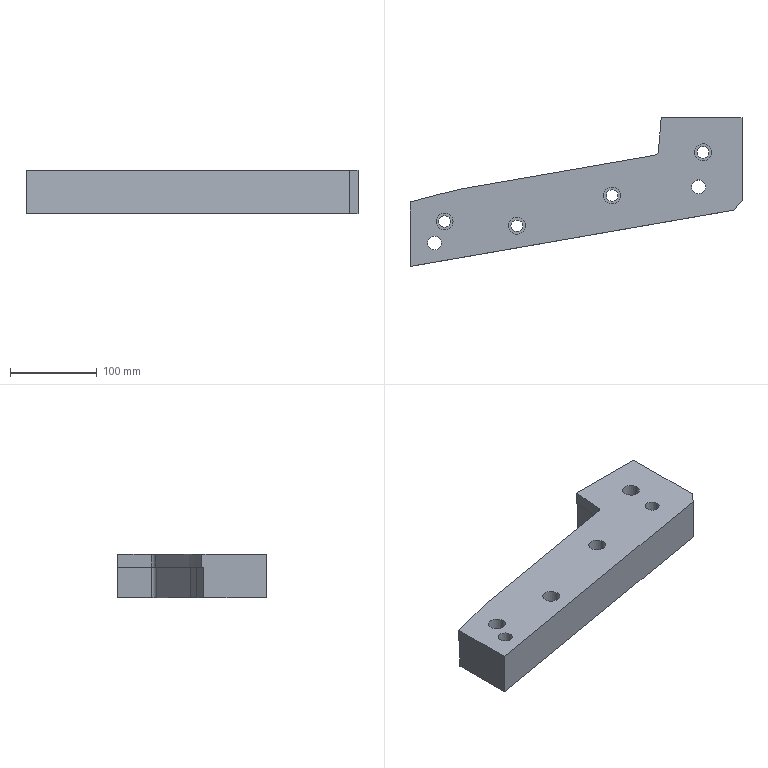Part | NX | features solid 2 | 1 solid | 31 faces | box 383.358 x 171.888 x 50 mm | volume 1583824 mm3 | plane 14 | cylinder 12 | spline 5 | commonest cylinder face diameters 13.5 x4 19.5 x4 16 x2 10 x1 14 x1
STEP:
#1=CARTESIAN_POINT('',(-1203.358,330.489,-15.));
#2=VERTEX_POINT('',#1);
#3=CARTESIAN_POINT('',(-1203.358,330.489,-50.));
#4=VERTEX_POINT('',#3);
#5=CARTESIAN_POINT('',(-1203.358,330.489,-32.5));
#6=DIRECTION('',(0.,0.,-1.));
#7=VECTOR('',#6,1000.);
#8=LINE('',#5,#7);
#9=EDGE_CURVE('',#2,#4,#8,.T.);
#10=ORIENTED_EDGE('',*,*,#9,.T.);
#11=CARTESIAN_POINT('',(-1203.358,258.112,-50.));
#12=VERTEX_POINT('',#11);
#13=CARTESIAN_POINT('',(-1203.358,307.899,-50.));
#14=DIRECTION('',(0.,-1.,0.));
#15=VECTOR('',#14,1000.);
#16=LINE('',#13,#15);
#17=EDGE_CURVE('',#4,#12,#16,.T.);
#18=ORIENTED_EDGE('',*,*,#17,.T.);
#19=CARTESIAN_POINT('',(-1203.358,258.112,0.));
#20=VERTEX_POINT('',#19);
#21=CARTESIAN_POINT('',(-1203.358,258.112,-50.));
#22=DIRECTION('',(0.,0.,1.));
#23=VECTOR('',#22,1000.);
#24=LINE('',#21,#23);
#25=EDGE_CURVE('',#12,#20,#24,.T.);
#26=ORIENTED_EDGE('',*,*,#25,.T.);
#27=CARTESIAN_POINT('',(-1203.358,332.538,0.));
#28=VERTEX_POINT('',#27);
#29=CARTESIAN_POINT('',(-1203.358,307.899,0.));
#30=DIRECTION('',(0.,-1.,0.));
#31=VECTOR('',#30,1000.);
#32=LINE('',#29,#31);
#33=EDGE_CURVE('',#28,#20,#32,.T.);
#34=ORIENTED_EDGE('',*,*,#33,.F.);
#35=CARTESIAN_POINT('',(-1203.358,332.538,-15.));
#36=VERTEX_POINT('',#35);
#37=CARTESIAN_POINT('',(-1203.358,332.538,0.));
#38=DIRECTION('',(0.,0.,1.));
#39=VECTOR('',#38,1000.);
#40=LINE('',#37,#39);
#41=EDGE_CURVE('',#28,#36,#40,.F.);
#42=ORIENTED_EDGE('',*,*,#41,.T.);
#43=CARTESIAN_POINT('',(-1203.358,390.837,-15.));
#44=DIRECTION('',(0.,-1.,0.));
#45=VECTOR('',#44,1000.);
#46=LINE('',#43,#45);
#47=EDGE_CURVE('',#2,#36,#46,.F.);
#48=ORIENTED_EDGE('',*,*,#47,.F.);
#49=EDGE_LOOP('',(#10,#18,#26,#34,#42,#48));
#50=FACE_BOUND('',#49,.T.);
#51=CARTESIAN_POINT('',(-1203.358,250.,0.));
#52=DIRECTION('',(1.,0.,0.));
#53=DIRECTION('',(0.,0.,-1.));
#54=AXIS2_PLACEMENT_3D('',#51,#52,#53);
#55=PLANE('',#54);
#56=ADVANCED_FACE('',(#50),#55,.F.);
#57=CARTESIAN_POINT('',(-1144.675,345.418,-15.));
#58=VERTEX_POINT('',#57);
#59=CARTESIAN_POINT('',(-1144.675,345.418,-50.));
#60=VERTEX_POINT('',#59);
#61=CARTESIAN_POINT('',(-1144.675,345.418,-65.));
#62=DIRECTION('',(0.,0.,-1.));
#63=VECTOR('',#62,1000.);
#64=LINE('',#61,#63);
#65=EDGE_CURVE('',#58,#60,#64,.T.);
#66=ORIENTED_EDGE('',*,*,#65,.F.);
#67=CARTESIAN_POINT('',(-920.081,384.447,-15.));
#68=VERTEX_POINT('',#67);
#69=CARTESIAN_POINT('',(-1144.675,345.418,-15.));
#70=CARTESIAN_POINT('',(-1107.244,351.927,-15.));
#71=CARTESIAN_POINT('',(-1051.098,361.701,-15.));
#72=CARTESIAN_POINT('',(-976.23,374.696,-15.));
#73=CARTESIAN_POINT('',(-938.808,381.26,-15.));
#74=CARTESIAN_POINT('',(-920.081,384.447,-15.));
#75=B_SPLINE_CURVE_WITH_KNOTS('',3,(#69,#70,#71,#72,#73,#74),.UNSPECIFIED.,.F.,.F.,(4,1,1,4),(0.07597,0.19,0.2469,0.3039),.UNSPECIFIED.);
#76=EDGE_CURVE('',#58,#68,#75,.T.);
#77=ORIENTED_EDGE('',*,*,#76,.T.);
#78=CARTESIAN_POINT('',(-920.081,384.446,-50.));
#79=VERTEX_POINT('',#78);
#80=CARTESIAN_POINT('',(-920.081,384.447,-32.5));
#81=DIRECTION('',(0.,0.,1.));
#82=VECTOR('',#81,1000.);
#83=LINE('',#80,#82);
#84=EDGE_CURVE('',#79,#68,#83,.T.);
#85=ORIENTED_EDGE('',*,*,#84,.F.);
#86=CARTESIAN_POINT('',(-920.081,384.447,-50.));
#87=CARTESIAN_POINT('',(-938.808,381.26,-50.));
#88=CARTESIAN_POINT('',(-976.23,374.696,-50.));
#89=CARTESIAN_POINT('',(-1051.098,361.701,-50.));
#90=CARTESIAN_POINT('',(-1107.244,351.927,-50.));
#91=CARTESIAN_POINT('',(-1144.675,345.418,-50.));
#92=B_SPLINE_CURVE_WITH_KNOTS('',3,(#86,#87,#88,#89,#90,#91),.UNSPECIFIED.,.F.,.F.,(4,1,1,4),(0.008531,0.06552,0.1225,0.2365),.UNSPECIFIED.);
#93=EDGE_CURVE('',#79,#60,#92,.T.);
#94=ORIENTED_EDGE('',*,*,#93,.T.);
#95=EDGE_LOOP('',(#66,#77,#85,#94));
#96=FACE_BOUND('',#95,.T.);
#97=CARTESIAN_POINT('',(-1144.675,345.418,-50.));
#98=CARTESIAN_POINT('',(-1144.675,345.418,-15.));
#99=CARTESIAN_POINT('',(-1107.243,351.928,-50.));
#100=CARTESIAN_POINT('',(-1107.243,351.928,-15.));
#101=CARTESIAN_POINT('',(-1051.094,361.702,-50.));
#102=CARTESIAN_POINT('',(-1051.094,361.702,-15.));
#103=CARTESIAN_POINT('',(-976.227,374.697,-50.));
#104=CARTESIAN_POINT('',(-976.227,374.697,-15.));
#105=CARTESIAN_POINT('',(-938.797,381.262,-50.));
#106=CARTESIAN_POINT('',(-938.797,381.262,-15.));
#107=CARTESIAN_POINT('',(-920.081,384.447,-50.));
#108=CARTESIAN_POINT('',(-920.081,384.447,-15.));
#109=B_SPLINE_SURFACE_WITH_KNOTS('',3,1,((#97,#98),(#99,#100),(#101,#102),(#103,#104),(#105,#106),(#107,#108)),.SURF_OF_LINEAR_EXTRUSION.,.F.,.F.,.F.,(4,1,1,4),(2,2),(0.3026,0.5897,0.7332,0.8768),(0.,1.),.UNSPECIFIED.);
#110=ADVANCED_FACE('',(#96),#109,.F.);
#111=CARTESIAN_POINT('',(-1086.75,305.,-50.));
#112=VERTEX_POINT('',#111);
#113=CARTESIAN_POINT('',(-1080.,305.,-50.));
#114=DIRECTION('',(0.,0.,-1.));
#115=DIRECTION('',(-1.,0.,0.));
#116=AXIS2_PLACEMENT_3D('',#113,#114,#115);
#117=CIRCLE('',#116,6.75);
#118=EDGE_CURVE('',#112,#112,#117,.T.);
#119=ORIENTED_EDGE('',*,*,#118,.F.);
#120=EDGE_LOOP('',(#119));
#121=FACE_BOUND('',#120,.T.);
#122=CARTESIAN_POINT('',(-976.75,340.,-50.));
#123=VERTEX_POINT('',#122);
#124=CARTESIAN_POINT('',(-970.,340.,-50.));
#125=DIRECTION('',(0.,0.,-1.));
#126=DIRECTION('',(-1.,0.,0.));
#127=AXIS2_PLACEMENT_3D('',#124,#125,#126);
#128=CIRCLE('',#127,6.75);
#129=EDGE_CURVE('',#123,#123,#128,.T.);
#130=ORIENTED_EDGE('',*,*,#129,.F.);
#131=EDGE_LOOP('',(#130));
#132=FACE_BOUND('',#131,.T.);
#133=CARTESIAN_POINT('',(-871.75,390.,-50.));
#134=VERTEX_POINT('',#133);
#135=CARTESIAN_POINT('',(-865.,390.,-50.));
#136=DIRECTION('',(0.,0.,-1.));
#137=DIRECTION('',(-1.,0.,0.));
#138=AXIS2_PLACEMENT_3D('',#135,#136,#137);
#139=CIRCLE('',#138,6.75);
#140=EDGE_CURVE('',#134,#134,#139,.T.);
#141=ORIENTED_EDGE('',*,*,#140,.F.);
#142=EDGE_LOOP('',(#141));
#143=FACE_BOUND('',#142,.T.);
#144=CARTESIAN_POINT('',(-1183.,285.,-50.));
#145=VERTEX_POINT('',#144);
#146=CARTESIAN_POINT('',(-1175.,285.,-50.));
#147=DIRECTION('',(0.,0.,-1.));
#148=DIRECTION('',(-1.,0.,0.));
#149=AXIS2_PLACEMENT_3D('',#146,#147,#148);
#150=CIRCLE('',#149,8.);
#151=EDGE_CURVE('',#145,#145,#150,.T.);
#152=ORIENTED_EDGE('',*,*,#151,.F.);
#153=EDGE_LOOP('',(#152));
#154=FACE_BOUND('',#153,.T.);
#155=CARTESIAN_POINT('',(-878.,350.,-50.));
#156=VERTEX_POINT('',#155);
#157=CARTESIAN_POINT('',(-870.,350.,-50.));
#158=DIRECTION('',(0.,0.,-1.));
#159=DIRECTION('',(-1.,0.,0.));
#160=AXIS2_PLACEMENT_3D('',#157,#158,#159);
#161=CIRCLE('',#160,8.);
#162=EDGE_CURVE('',#156,#156,#161,.T.);
#163=ORIENTED_EDGE('',*,*,#162,.F.);
#164=EDGE_LOOP('',(#163));
#165=FACE_BOUND('',#164,.T.);
#166=CARTESIAN_POINT('',(-1170.108,310.,-50.));
#167=VERTEX_POINT('',#166);
#168=CARTESIAN_POINT('',(-1163.358,310.,-50.));
#169=DIRECTION('',(0.,0.,-1.));
#170=DIRECTION('',(-1.,0.,0.));
#171=AXIS2_PLACEMENT_3D('',#168,#169,#170);
#172=CIRCLE('',#171,6.75);
#173=EDGE_CURVE('',#167,#167,#172,.T.);
#174=ORIENTED_EDGE('',*,*,#173,.F.);
#175=EDGE_LOOP('',(#174));
#176=FACE_BOUND('',#175,.T.);
#177=ORIENTED_EDGE('',*,*,#17,.F.);
#178=CARTESIAN_POINT('',(-1173.872,338.321,-50.));
#179=VERTEX_POINT('',#178);
#180=CARTESIAN_POINT('',(-1173.872,338.321,-50.));
#181=CARTESIAN_POINT('',(-1183.662,335.564,-50.));
#182=CARTESIAN_POINT('',(-1193.43,332.709,-50.));
#183=CARTESIAN_POINT('',(-1203.358,330.489,-50.));
#184=B_SPLINE_CURVE_WITH_KNOTS('',3,(#180,#181,#182,#183),.UNSPECIFIED.,.F.,.F.,(4,4),(0.,0.03051),.UNSPECIFIED.);
#185=EDGE_CURVE('',#179,#4,#184,.T.);
#186=ORIENTED_EDGE('',*,*,#185,.F.);
#187=CARTESIAN_POINT('',(-1173.872,338.321,-50.));
#188=CARTESIAN_POINT('',(-1164.227,341.036,-50.));
#189=CARTESIAN_POINT('',(-1154.52,343.549,-50.));
#190=CARTESIAN_POINT('',(-1144.675,345.418,-50.));
#191=B_SPLINE_CURVE_WITH_KNOTS('',3,(#187,#188,#189,#190),.UNSPECIFIED.,.F.,.F.,(4,4),(0.,0.03006),.UNSPECIFIED.);
#192=EDGE_CURVE('',#179,#60,#191,.T.);
#193=ORIENTED_EDGE('',*,*,#192,.T.);
#194=ORIENTED_EDGE('',*,*,#93,.F.);
#195=CARTESIAN_POINT('',(-914.658,390.663,-50.));
#196=VERTEX_POINT('',#195);
#197=CARTESIAN_POINT('',(-921.632,391.273,-50.));
#198=DIRECTION('',(0.,0.,1.));
#199=DIRECTION('',(1.,0.,0.));
#200=AXIS2_PLACEMENT_3D('',#197,#198,#199);
#201=CIRCLE('',#200,7.);
#202=EDGE_CURVE('',#79,#196,#201,.T.);
#203=ORIENTED_EDGE('',*,*,#202,.T.);
#204=CARTESIAN_POINT('',(-911.217,430.,-50.));
#205=VERTEX_POINT('',#204);
#206=CARTESIAN_POINT('',(-914.658,390.663,-50.));
#207=DIRECTION('',(0.08716,0.9962,0.));
#208=VECTOR('',#207,1000.);
#209=LINE('',#206,#208);
#210=EDGE_CURVE('',#196,#205,#209,.T.);
#211=ORIENTED_EDGE('',*,*,#210,.T.);
#212=CARTESIAN_POINT('',(-820.,430.,-50.));
#213=VERTEX_POINT('',#212);
#214=CARTESIAN_POINT('',(-752.827,430.,-50.));
#215=DIRECTION('',(-1.,0.,0.));
#216=VECTOR('',#215,1000.);
#217=LINE('',#214,#216);
#218=EDGE_CURVE('',#205,#213,#217,.F.);
#219=ORIENTED_EDGE('',*,*,#218,.T.);
#220=CARTESIAN_POINT('',(-820.,334.782,-50.));
#221=VERTEX_POINT('',#220);
#222=CARTESIAN_POINT('',(-820.,410.,-50.));
#223=DIRECTION('',(0.,-1.,0.));
#224=VECTOR('',#223,1000.);
#225=LINE('',#222,#224);
#226=EDGE_CURVE('',#213,#221,#225,.T.);
#227=ORIENTED_EDGE('',*,*,#226,.T.);
#228=CARTESIAN_POINT('',(-829.852,323.069,-50.));
#229=VERTEX_POINT('',#228);
#230=CARTESIAN_POINT('',(-916.896,219.58,-50.));
#231=DIRECTION('',(-0.6437,-0.7653,0.));
#232=VECTOR('',#231,1000.);
#233=LINE('',#230,#232);
#234=EDGE_CURVE('',#221,#229,#233,.T.);
#235=ORIENTED_EDGE('',*,*,#234,.T.);
#236=CARTESIAN_POINT('',(-1250.,250.,-50.));
#237=DIRECTION('',(0.9852,0.1713,0.));
#238=VECTOR('',#237,1000.);
#239=LINE('',#236,#238);
#240=EDGE_CURVE('',#12,#229,#239,.T.);
#241=ORIENTED_EDGE('',*,*,#240,.F.);
#242=EDGE_LOOP('',(#177,#186,#193,#194,#203,#211,#219,#227,#235,#241));
#243=FACE_BOUND('',#242,.T.);
#244=CARTESIAN_POINT('',(-1021.9,307.899,-50.));
#245=DIRECTION('',(0.,0.,-1.));
#246=DIRECTION('',(-1.,0.,0.));
#247=AXIS2_PLACEMENT_3D('',#244,#245,#246);
#248=PLANE('',#247);
#249=ADVANCED_FACE('',(#121,#132,#143,#154,#165,#176,#243),#248,.T.);
#250=CARTESIAN_POINT('',(-878.,350.,0.));
#251=VERTEX_POINT('',#250);
#252=CARTESIAN_POINT('',(-870.,350.,0.));
#253=DIRECTION('',(0.,0.,-1.));
#254=DIRECTION('',(-1.,0.,0.));
#255=AXIS2_PLACEMENT_3D('',#252,#253,#254);
#256=CIRCLE('',#255,8.);
#257=EDGE_CURVE('',#251,#251,#256,.T.);
#258=ORIENTED_EDGE('',*,*,#257,.F.);
#259=EDGE_LOOP('',(#258));
#260=FACE_BOUND('',#259,.T.);
#261=ORIENTED_EDGE('',*,*,#162,.T.);
#262=EDGE_LOOP('',(#261));
#263=FACE_BOUND('',#262,.T.);
#264=CARTESIAN_POINT('',(-870.,350.,0.));
#265=DIRECTION('',(0.,0.,-1.));
#266=DIRECTION('',(-1.,0.,0.));
#267=AXIS2_PLACEMENT_3D('',#264,#265,#266);
#268=CYLINDRICAL_SURFACE('',#267,8.);
#269=ADVANCED_FACE('',(#260,#263),#268,.F.);
#270=CARTESIAN_POINT('',(-1183.,285.,0.));
#271=VERTEX_POINT('',#270);
#272=CARTESIAN_POINT('',(-1175.,285.,0.));
#273=DIRECTION('',(0.,0.,-1.));
#274=DIRECTION('',(-1.,0.,0.));
#275=AXIS2_PLACEMENT_3D('',#272,#273,#274);
#276=CIRCLE('',#275,8.);
#277=EDGE_CURVE('',#271,#271,#276,.T.);
#278=ORIENTED_EDGE('',*,*,#277,.F.);
#279=EDGE_LOOP('',(#278));
#280=FACE_BOUND('',#279,.T.);
#281=ORIENTED_EDGE('',*,*,#151,.T.);
#282=EDGE_LOOP('',(#281));
#283=FACE_BOUND('',#282,.T.);
#284=CARTESIAN_POINT('',(-1175.,285.,0.));
#285=DIRECTION('',(0.,0.,-1.));
#286=DIRECTION('',(-1.,0.,0.));
#287=AXIS2_PLACEMENT_3D('',#284,#285,#286);
#288=CYLINDRICAL_SURFACE('',#287,8.);
#289=ADVANCED_FACE('',(#280,#283),#288,.F.);
#290=CARTESIAN_POINT('',(-874.75,390.,0.));
#291=VERTEX_POINT('',#290);
#292=CARTESIAN_POINT('',(-865.,390.,0.));
#293=DIRECTION('',(0.,0.,-1.));
#294=DIRECTION('',(-1.,0.,0.));
#295=AXIS2_PLACEMENT_3D('',#292,#293,#294);
#296=CIRCLE('',#295,9.75);
#297=EDGE_CURVE('',#291,#291,#296,.T.);
#298=ORIENTED_EDGE('',*,*,#297,.F.);
#299=EDGE_LOOP('',(#298));
#300=FACE_BOUND('',#299,.T.);
#301=CARTESIAN_POINT('',(-874.75,390.,-25.));
#302=VERTEX_POINT('',#301);
#303=CARTESIAN_POINT('',(-865.,390.,-25.));
#304=DIRECTION('',(0.,0.,-1.));
#305=DIRECTION('',(-1.,0.,0.));
#306=AXIS2_PLACEMENT_3D('',#303,#304,#305);
#307=CIRCLE('',#306,9.75);
#308=EDGE_CURVE('',#302,#302,#307,.T.);
#309=ORIENTED_EDGE('',*,*,#308,.T.);
#310=EDGE_LOOP('',(#309));
#311=FACE_BOUND('',#310,.T.);
#312=CARTESIAN_POINT('',(-865.,390.,0.));
#313=DIRECTION('',(0.,0.,-1.));
#314=DIRECTION('',(-1.,0.,0.));
#315=AXIS2_PLACEMENT_3D('',#312,#313,#314);
#316=CYLINDRICAL_SURFACE('',#315,9.75);
#317=ADVANCED_FACE('',(#300,#311),#316,.F.);
#318=CARTESIAN_POINT('',(-979.75,340.,0.));
#319=VERTEX_POINT('',#318);
#320=CARTESIAN_POINT('',(-970.,340.,0.));
#321=DIRECTION('',(0.,0.,-1.));
#322=DIRECTION('',(-1.,0.,0.));
#323=AXIS2_PLACEMENT_3D('',#320,#321,#322);
#324=CIRCLE('',#323,9.75);
#325=EDGE_CURVE('',#319,#319,#324,.T.);
#326=ORIENTED_EDGE('',*,*,#325,.F.);
#327=EDGE_LOOP('',(#326));
#328=FACE_BOUND('',#327,.T.);
#329=CARTESIAN_POINT('',(-979.75,340.,-25.));
#330=VERTEX_POINT('',#329);
#331=CARTESIAN_POINT('',(-970.,340.,-25.));
#332=DIRECTION('',(0.,0.,-1.));
#333=DIRECTION('',(-1.,0.,0.));
#334=AXIS2_PLACEMENT_3D('',#331,#332,#333);
#335=CIRCLE('',#334,9.75);
#336=EDGE_CURVE('',#330,#330,#335,.T.);
#337=ORIENTED_EDGE('',*,*,#336,.T.);
#338=EDGE_LOOP('',(#337));
#339=FACE_BOUND('',#338,.T.);
#340=CARTESIAN_POINT('',(-970.,340.,0.));
#341=DIRECTION('',(0.,0.,-1.));
#342=DIRECTION('',(-1.,0.,0.));
#343=AXIS2_PLACEMENT_3D('',#340,#341,#342);
#344=CYLINDRICAL_SURFACE('',#343,9.75);
#345=ADVANCED_FACE('',(#328,#339),#344,.F.);
#346=CARTESIAN_POINT('',(-1089.75,305.,0.));
#347=VERTEX_POINT('',#346);
#348=CARTESIAN_POINT('',(-1080.,305.,0.));
#349=DIRECTION('',(0.,0.,-1.));
#350=DIRECTION('',(-1.,0.,0.));
#351=AXIS2_PLACEMENT_3D('',#348,#349,#350);
#352=CIRCLE('',#351,9.75);
#353=EDGE_CURVE('',#347,#347,#352,.T.);
#354=ORIENTED_EDGE('',*,*,#353,.F.);
#355=EDGE_LOOP('',(#354));
#356=FACE_BOUND('',#355,.T.);
#357=CARTESIAN_POINT('',(-1089.75,305.,-25.));
#358=VERTEX_POINT('',#357);
#359=CARTESIAN_POINT('',(-1080.,305.,-25.));
#360=DIRECTION('',(0.,0.,-1.));
#361=DIRECTION('',(-1.,0.,0.));
#362=AXIS2_PLACEMENT_3D('',#359,#360,#361);
#363=CIRCLE('',#362,9.75);
#364=EDGE_CURVE('',#358,#358,#363,.T.);
#365=ORIENTED_EDGE('',*,*,#364,.T.);
#366=EDGE_LOOP('',(#365));
#367=FACE_BOUND('',#366,.T.);
#368=CARTESIAN_POINT('',(-1080.,305.,0.));
#369=DIRECTION('',(0.,0.,-1.));
#370=DIRECTION('',(-1.,0.,0.));
#371=AXIS2_PLACEMENT_3D('',#368,#369,#370);
#372=CYLINDRICAL_SURFACE('',#371,9.75);
#373=ADVANCED_FACE('',(#356,#367),#372,.F.);
#374=CARTESIAN_POINT('',(-1145.033,347.385,-15.));
#375=VERTEX_POINT('',#374);
#376=CARTESIAN_POINT('',(-920.475,386.408,-15.));
#377=VERTEX_POINT('',#376);
#378=CARTESIAN_POINT('',(-1145.033,347.385,-15.));
#379=CARTESIAN_POINT('',(-1107.608,353.894,-15.));
#380=CARTESIAN_POINT('',(-1051.471,363.666,-15.));
#381=CARTESIAN_POINT('',(-976.616,376.659,-15.));
#382=CARTESIAN_POINT('',(-939.199,383.222,-15.));
#383=CARTESIAN_POINT('',(-920.475,386.408,-15.));
#384=B_SPLINE_CURVE_WITH_KNOTS('',3,(#378,#379,#380,#381,#382,#383),.UNSPECIFIED.,.F.,.F.,(4,1,1,4),(0.637,0.7509,0.8079,0.8649),.UNSPECIFIED.);
#385=EDGE_CURVE('',#375,#377,#384,.T.);
#386=ORIENTED_EDGE('',*,*,#385,.F.);
#387=CARTESIAN_POINT('',(-1145.033,347.385,0.));
#388=VERTEX_POINT('',#387);
#389=CARTESIAN_POINT('',(-1145.033,347.385,-7.5));
#390=DIRECTION('',(0.,0.,1.));
#391=VECTOR('',#390,1000.);
#392=LINE('',#389,#391);
#393=EDGE_CURVE('',#375,#388,#392,.T.);
#394=ORIENTED_EDGE('',*,*,#393,.T.);
#395=CARTESIAN_POINT('',(-920.475,386.408,0.));
#396=VERTEX_POINT('',#395);
#397=CARTESIAN_POINT('',(-1323.576,316.335,0.));
#398=CARTESIAN_POINT('',(-1303.952,319.748,0.));
#399=CARTESIAN_POINT('',(-1284.328,323.16,0.));
#400=CARTESIAN_POINT('',(-1264.704,326.573,0.));
#401=CARTESIAN_POINT('',(-1233.889,331.932,0.));
#402=CARTESIAN_POINT('',(-1172.258,342.651,0.));
#403=CARTESIAN_POINT('',(-1095.22,356.049,0.));
#404=CARTESIAN_POINT('',(-1033.589,366.767,0.));
#405=CARTESIAN_POINT('',(-987.365,374.804,0.));
#406=CARTESIAN_POINT('',(-948.847,381.509,0.));
#407=CARTESIAN_POINT('',(-923.808,385.853,0.));
#408=CARTESIAN_POINT('',(-914.109,387.486,0.));
#409=CARTESIAN_POINT('',(-912.091,387.827,0.));
#410=CARTESIAN_POINT('',(-911.971,387.848,0.));
#411=CARTESIAN_POINT('',(-911.79,387.876,0.));
#412=CARTESIAN_POINT('',(-911.394,387.917,0.));
#413=CARTESIAN_POINT('',(-910.546,388.022,0.));
#414=CARTESIAN_POINT('',(-908.847,388.221,0.));
#415=CARTESIAN_POINT('',(-906.42,388.511,0.));
#416=CARTESIAN_POINT('',(-903.994,388.799,0.));
#417=CARTESIAN_POINT('',(-902.295,389.001,0.));
#418=CARTESIAN_POINT('',(-901.446,389.101,0.));
#419=CARTESIAN_POINT('',(-901.052,389.148,0.));
#420=CARTESIAN_POINT('',(-900.87,389.17,0.));
#421=CARTESIAN_POINT('',(-900.748,389.184,0.));
#422=CARTESIAN_POINT('',(-899.68,389.239,0.));
#423=CARTESIAN_POINT('',(-897.973,389.35,0.));
#424=CARTESIAN_POINT('',(-896.023,389.486,0.));
#425=CARTESIAN_POINT('',(-894.456,389.561,0.));
#426=CARTESIAN_POINT('',(-892.989,389.903,0.));
#427=CARTESIAN_POINT('',(-891.495,390.907,0.));
#428=CARTESIAN_POINT('',(-890.458,392.378,0.));
#429=CARTESIAN_POINT('',(-890.077,393.863,0.));
#430=CARTESIAN_POINT('',(-889.825,397.101,0.));
#431=CARTESIAN_POINT('',(-889.362,402.393,0.));
#432=CARTESIAN_POINT('',(-888.928,407.354,0.));
#433=CARTESIAN_POINT('',(-888.696,410.,0.));
#434=CARTESIAN_POINT('',(-886.96,429.843,0.));
#435=CARTESIAN_POINT('',(-885.224,449.685,0.));
#436=CARTESIAN_POINT('',(-883.488,469.528,0.));
#437=B_SPLINE_CURVE_WITH_KNOTS('',3,(#397,#398,#399,#400,#401,#402,#403,#404,#405,#406,#407,#408,#409,#410,#411,#412,#413,#414,#415,#416,#417,#418,#419,#420,#421,#422,#423,#424,#425,#426,#427,#428,#429,#430,#431,#432,#433,#434,#435,#436),.UNSPECIFIED.,.F.,.F.,(4,3,1,1,1,1,1,1,1,1,1,1,1,1,1,1,1,1,1,1,1,1,1,1,1,1,1,1,1,1,1,1,3,4),(-0.15,0.,0.2355,0.4711,0.5889,0.7066,0.8244,0.8833,0.898,0.8985,0.8987,0.8989,0.8999,0.9017,0.9054,0.9127,0.9201,0.9238,0.9256,0.9265,0.9268,0.927,0.9275,0.9348,0.9399,0.9422,0.9466,0.9511,0.9555,0.96,0.9625,0.98,1.,1.15),.UNSPECIFIED.);
#438=EDGE_CURVE('',#388,#396,#437,.T.);
#439=ORIENTED_EDGE('',*,*,#438,.T.);
#440=CARTESIAN_POINT('',(-920.475,386.408,-7.5));
#441=DIRECTION('',(0.,0.,1.));
#442=VECTOR('',#441,1000.);
#443=LINE('',#440,#442);
#444=EDGE_CURVE('',#377,#396,#443,.T.);
#445=ORIENTED_EDGE('',*,*,#444,.F.);
#446=EDGE_LOOP('',(#386,#394,#439,#445));
#447=FACE_BOUND('',#446,.T.);
#448=CARTESIAN_POINT('',(-1145.033,347.385,-15.));
#449=CARTESIAN_POINT('',(-1145.033,347.385,0.));
#450=CARTESIAN_POINT('',(-1107.608,353.894,-15.));
#451=CARTESIAN_POINT('',(-1107.608,353.894,0.));
#452=CARTESIAN_POINT('',(-1051.471,363.666,-15.));
#453=CARTESIAN_POINT('',(-1051.471,363.666,0.));
#454=CARTESIAN_POINT('',(-976.616,376.659,-15.));
#455=CARTESIAN_POINT('',(-976.616,376.659,0.));
#456=CARTESIAN_POINT('',(-939.199,383.222,-15.));
#457=CARTESIAN_POINT('',(-939.199,383.222,0.));
#458=CARTESIAN_POINT('',(-920.475,386.408,-15.));
#459=CARTESIAN_POINT('',(-920.475,386.408,0.));
#460=B_SPLINE_SURFACE_WITH_KNOTS('',3,1,((#448,#449),(#450,#451),(#452,#453),(#454,#455),(#456,#457),(#458,#459)),.SURF_OF_LINEAR_EXTRUSION.,.F.,.F.,.F.,(4,1,1,4),(2,2),(0.3049,0.591,0.734,0.8771),(0.,1.),.UNSPECIFIED.);
#461=ADVANCED_FACE('',(#447),#460,.F.);
#462=CARTESIAN_POINT('',(-916.651,390.837,-15.));
#463=VERTEX_POINT('',#462);
#464=CARTESIAN_POINT('',(-913.224,430.,-15.));
#465=VERTEX_POINT('',#464);
#466=CARTESIAN_POINT('',(-916.651,390.837,-15.));
#467=DIRECTION('',(0.08716,0.9962,0.));
#468=VECTOR('',#467,1000.);
#469=LINE('',#466,#468);
#470=EDGE_CURVE('',#463,#465,#469,.T.);
#471=ORIENTED_EDGE('',*,*,#470,.F.);
#472=CARTESIAN_POINT('',(-916.651,390.837,0.));
#473=VERTEX_POINT('',#472);
#474=CARTESIAN_POINT('',(-916.651,390.837,-50.));
#475=DIRECTION('',(0.,0.,1.));
#476=VECTOR('',#475,1000.);
#477=LINE('',#474,#476);
#478=EDGE_CURVE('',#463,#473,#477,.T.);
#479=ORIENTED_EDGE('',*,*,#478,.T.);
#480=CARTESIAN_POINT('',(-913.224,430.,0.));
#481=VERTEX_POINT('',#480);
#482=CARTESIAN_POINT('',(-916.651,390.837,0.));
#483=DIRECTION('',(0.08716,0.9962,0.));
#484=VECTOR('',#483,1000.);
#485=LINE('',#482,#484);
#486=EDGE_CURVE('',#473,#481,#485,.T.);
#487=ORIENTED_EDGE('',*,*,#486,.T.);
#488=CARTESIAN_POINT('',(-913.224,430.,-50.));
#489=DIRECTION('',(0.,0.,1.));
#490=VECTOR('',#489,1000.);
#491=LINE('',#488,#490);
#492=EDGE_CURVE('',#465,#481,#491,.T.);
#493=ORIENTED_EDGE('',*,*,#492,.F.);
#494=EDGE_LOOP('',(#471,#479,#487,#493));
#495=FACE_BOUND('',#494,.T.);
#496=CARTESIAN_POINT('',(-916.651,390.837,-50.));
#497=DIRECTION('',(0.9962,-0.08716,0.));
#498=DIRECTION('',(0.08716,0.9962,0.));
#499=AXIS2_PLACEMENT_3D('',#496,#497,#498);
#500=PLANE('',#499);
#501=ADVANCED_FACE('',(#495),#500,.F.);
#502=CARTESIAN_POINT('',(-921.632,391.273,-15.));
#503=DIRECTION('',(0.,0.,1.));
#504=DIRECTION('',(1.,0.,0.));
#505=AXIS2_PLACEMENT_3D('',#502,#503,#504);
#506=CIRCLE('',#505,5.);
#507=EDGE_CURVE('',#377,#463,#506,.T.);
#508=ORIENTED_EDGE('',*,*,#507,.F.);
#509=ORIENTED_EDGE('',*,*,#444,.T.);
#510=CARTESIAN_POINT('',(-921.632,391.273,0.));
#511=DIRECTION('',(0.,0.,1.));
#512=DIRECTION('',(1.,0.,0.));
#513=AXIS2_PLACEMENT_3D('',#510,#511,#512);
#514=CIRCLE('',#513,5.);
#515=EDGE_CURVE('',#396,#473,#514,.T.);
#516=ORIENTED_EDGE('',*,*,#515,.T.);
#517=ORIENTED_EDGE('',*,*,#478,.F.);
#518=EDGE_LOOP('',(#508,#509,#516,#517));
#519=FACE_BOUND('',#518,.T.);
#520=CARTESIAN_POINT('',(-921.632,391.273,-50.));
#521=DIRECTION('',(0.,0.,1.));
#522=DIRECTION('',(1.,0.,0.));
#523=AXIS2_PLACEMENT_3D('',#520,#521,#522);
#524=CYLINDRICAL_SURFACE('',#523,5.);
#525=ADVANCED_FACE('',(#519),#524,.F.);
#526=CARTESIAN_POINT('',(-1145.033,347.385,-15.));
#527=CARTESIAN_POINT('',(-1149.963,346.45,-15.));
#528=CARTESIAN_POINT('',(-1159.758,344.299,-15.));
#529=CARTESIAN_POINT('',(-1179.117,338.99,-15.));
#530=CARTESIAN_POINT('',(-1193.571,334.727,-15.));
#531=CARTESIAN_POINT('',(-1203.358,332.538,-15.));
#532=B_SPLINE_CURVE_WITH_KNOTS('',3,(#526,#527,#528,#529,#530,#531),.UNSPECIFIED.,.F.,.F.,(4,1,1,4),(0.1827,0.1978,0.2128,0.2429),.UNSPECIFIED.);
#533=EDGE_CURVE('',#36,#375,#532,.F.);
#534=ORIENTED_EDGE('',*,*,#533,.T.);
#535=ORIENTED_EDGE('',*,*,#385,.T.);
#536=ORIENTED_EDGE('',*,*,#507,.T.);
#537=ORIENTED_EDGE('',*,*,#470,.T.);
#538=CARTESIAN_POINT('',(-911.217,430.,-15.));
#539=VERTEX_POINT('',#538);
#540=CARTESIAN_POINT('',(-872.888,430.,-15.));
#541=DIRECTION('',(-1.,0.,0.));
#542=VECTOR('',#541,1000.);
#543=LINE('',#540,#542);
#544=EDGE_CURVE('',#465,#539,#543,.F.);
#545=ORIENTED_EDGE('',*,*,#544,.T.);
#546=CARTESIAN_POINT('',(-914.658,390.663,-15.));
#547=VERTEX_POINT('',#546);
#548=CARTESIAN_POINT('',(-914.658,390.663,-15.));
#549=DIRECTION('',(0.08716,0.9962,0.));
#550=VECTOR('',#549,1000.);
#551=LINE('',#548,#550);
#552=EDGE_CURVE('',#547,#539,#551,.T.);
#553=ORIENTED_EDGE('',*,*,#552,.F.);
#554=CARTESIAN_POINT('',(-921.632,391.273,-15.));
#555=DIRECTION('',(0.,0.,-1.));
#556=DIRECTION('',(-1.,0.,0.));
#557=AXIS2_PLACEMENT_3D('',#554,#555,#556);
#558=CIRCLE('',#557,7.);
#559=EDGE_CURVE('',#68,#547,#558,.F.);
#560=ORIENTED_EDGE('',*,*,#559,.F.);
#561=ORIENTED_EDGE('',*,*,#76,.F.);
#562=CARTESIAN_POINT('',(-1173.872,338.321,-15.));
#563=VERTEX_POINT('',#562);
#564=CARTESIAN_POINT('',(-1173.872,338.321,-15.));
#565=CARTESIAN_POINT('',(-1164.228,341.036,-15.));
#566=CARTESIAN_POINT('',(-1154.519,343.549,-15.));
#567=CARTESIAN_POINT('',(-1144.675,345.418,-15.));
#568=B_SPLINE_CURVE_WITH_KNOTS('',3,(#564,#565,#566,#567),.UNSPECIFIED.,.F.,.F.,(4,4),(0.1211,0.1511),.UNSPECIFIED.);
#569=EDGE_CURVE('',#563,#58,#568,.T.);
#570=ORIENTED_EDGE('',*,*,#569,.F.);
#571=CARTESIAN_POINT('',(-1173.872,338.321,-15.));
#572=CARTESIAN_POINT('',(-1183.662,335.564,-15.));
#573=CARTESIAN_POINT('',(-1193.43,332.709,-15.));
#574=CARTESIAN_POINT('',(-1203.358,330.489,-15.));
#575=B_SPLINE_CURVE_WITH_KNOTS('',3,(#571,#572,#573,#574),.UNSPECIFIED.,.F.,.F.,(4,4),(0.,0.03051),.UNSPECIFIED.);
#576=EDGE_CURVE('',#563,#2,#575,.T.);
#577=ORIENTED_EDGE('',*,*,#576,.T.);
#578=ORIENTED_EDGE('',*,*,#47,.T.);
#579=EDGE_LOOP('',(#534,#535,#536,#537,#545,#553,#560,#561,#570,#577,#578));
#580=FACE_BOUND('',#579,.T.);
#581=CARTESIAN_POINT('',(-916.651,390.837,-15.));
#582=DIRECTION('',(0.,0.,-1.));
#583=DIRECTION('',(0.08716,0.9962,0.));
#584=AXIS2_PLACEMENT_3D('',#581,#582,#583);
#585=PLANE('',#584);
#586=ADVANCED_FACE('',(#580),#585,.T.);
#587=ORIENTED_EDGE('',*,*,#25,.F.);
#588=ORIENTED_EDGE('',*,*,#240,.T.);
#589=CARTESIAN_POINT('',(-829.852,323.069,0.));
#590=VERTEX_POINT('',#589);
#591=CARTESIAN_POINT('',(-829.852,323.069,0.));
#592=DIRECTION('',(0.,0.,1.));
#593=VECTOR('',#592,1000.);
#594=LINE('',#591,#593);
#595=EDGE_CURVE('',#229,#590,#594,.T.);
#596=ORIENTED_EDGE('',*,*,#595,.T.);
#597=CARTESIAN_POINT('',(-1250.,250.,0.));
#598=DIRECTION('',(0.9852,0.1713,0.));
#599=VECTOR('',#598,1000.);
#600=LINE('',#597,#599);
#601=EDGE_CURVE('',#20,#590,#600,.T.);
#602=ORIENTED_EDGE('',*,*,#601,.F.);
#603=EDGE_LOOP('',(#587,#588,#596,#602));
#604=FACE_BOUND('',#603,.T.);
#605=CARTESIAN_POINT('',(-1250.,250.,-50.));
#606=DIRECTION('',(0.1713,-0.9852,0.));
#607=DIRECTION('',(0.9852,0.1713,0.));
#608=AXIS2_PLACEMENT_3D('',#605,#606,#607);
#609=PLANE('',#608);
#610=ADVANCED_FACE('',(#604),#609,.T.);
#611=CARTESIAN_POINT('',(-820.,430.,0.));
#612=VERTEX_POINT('',#611);
#613=CARTESIAN_POINT('',(-820.,430.,-50.));
#614=DIRECTION('',(0.,0.,-1.));
#615=VECTOR('',#614,1000.);
#616=LINE('',#613,#615);
#617=EDGE_CURVE('',#213,#612,#616,.F.);
#618=ORIENTED_EDGE('',*,*,#617,.F.);
#619=ORIENTED_EDGE('',*,*,#218,.F.);
#620=CARTESIAN_POINT('',(-911.217,430.,-50.));
#621=DIRECTION('',(0.,0.,1.));
#622=VECTOR('',#621,1000.);
#623=LINE('',#620,#622);
#624=EDGE_CURVE('',#205,#539,#623,.T.);
#625=ORIENTED_EDGE('',*,*,#624,.T.);
#626=ORIENTED_EDGE('',*,*,#544,.F.);
#627=ORIENTED_EDGE('',*,*,#492,.T.);
#628=CARTESIAN_POINT('',(-752.827,430.,0.));
#629=DIRECTION('',(-1.,0.,0.));
#630=VECTOR('',#629,1000.);
#631=LINE('',#628,#630);
#632=EDGE_CURVE('',#481,#612,#631,.F.);
#633=ORIENTED_EDGE('',*,*,#632,.T.);
#634=EDGE_LOOP('',(#618,#619,#625,#626,#627,#633));
#635=FACE_BOUND('',#634,.T.);
#636=CARTESIAN_POINT('',(-752.827,430.,-50.));
#637=DIRECTION('',(0.,1.,0.));
#638=DIRECTION('',(-1.,0.,0.));
#639=AXIS2_PLACEMENT_3D('',#636,#637,#638);
#640=PLANE('',#639);
#641=ADVANCED_FACE('',(#635),#640,.T.);
#642=ORIENTED_EDGE('',*,*,#595,.F.);
#643=ORIENTED_EDGE('',*,*,#234,.F.);
#644=CARTESIAN_POINT('',(-820.,334.782,0.));
#645=VERTEX_POINT('',#644);
#646=CARTESIAN_POINT('',(-820.,334.782,-50.));
#647=DIRECTION('',(0.,0.,-1.));
#648=VECTOR('',#647,1000.);
#649=LINE('',#646,#648);
#650=EDGE_CURVE('',#645,#221,#649,.T.);
#651=ORIENTED_EDGE('',*,*,#650,.F.);
#652=CARTESIAN_POINT('',(-829.852,323.069,0.));
#653=DIRECTION('',(0.6437,0.7653,0.));
#654=VECTOR('',#653,1000.);
#655=LINE('',#652,#654);
#656=EDGE_CURVE('',#590,#645,#655,.T.);
#657=ORIENTED_EDGE('',*,*,#656,.F.);
#658=EDGE_LOOP('',(#642,#643,#651,#657));
#659=FACE_BOUND('',#658,.T.);
#660=CARTESIAN_POINT('',(-829.852,323.069,-50.));
#661=DIRECTION('',(0.7653,-0.6437,0.));
#662=DIRECTION('',(0.6437,0.7653,0.));
#663=AXIS2_PLACEMENT_3D('',#660,#661,#662);
#664=PLANE('',#663);
#665=ADVANCED_FACE('',(#659),#664,.T.);
#666=ORIENTED_EDGE('',*,*,#650,.T.);
#667=ORIENTED_EDGE('',*,*,#226,.F.);
#668=ORIENTED_EDGE('',*,*,#617,.T.);
#669=CARTESIAN_POINT('',(-820.,410.,0.));
#670=DIRECTION('',(0.,-1.,0.));
#671=VECTOR('',#670,1000.);
#672=LINE('',#669,#671);
#673=EDGE_CURVE('',#612,#645,#672,.T.);
#674=ORIENTED_EDGE('',*,*,#673,.T.);
#675=EDGE_LOOP('',(#666,#667,#668,#674));
#676=FACE_BOUND('',#675,.T.);
#677=CARTESIAN_POINT('',(-820.,410.,-50.));
#678=DIRECTION('',(-1.,0.,0.));
#679=DIRECTION('',(0.,-1.,0.));
#680=AXIS2_PLACEMENT_3D('',#677,#678,#679);
#681=PLANE('',#680);
#682=ADVANCED_FACE('',(#676),#681,.F.);
#683=ORIENTED_EDGE('',*,*,#438,.F.);
#684=CARTESIAN_POINT('',(-1145.033,347.385,0.));
#685=CARTESIAN_POINT('',(-1149.954,346.452,0.));
#686=CARTESIAN_POINT('',(-1159.739,344.303,0.));
#687=CARTESIAN_POINT('',(-1179.108,338.993,0.));
#688=CARTESIAN_POINT('',(-1193.576,334.726,0.));
#689=CARTESIAN_POINT('',(-1203.358,332.538,0.));
#690=B_SPLINE_CURVE_WITH_KNOTS('',3,(#684,#685,#686,#687,#688,#689),.UNSPECIFIED.,.F.,.F.,(4,1,1,4),(0.2084,0.2234,0.2385,0.2685),.UNSPECIFIED.);
#691=EDGE_CURVE('',#388,#28,#690,.T.);
#692=ORIENTED_EDGE('',*,*,#691,.T.);
#693=ORIENTED_EDGE('',*,*,#33,.T.);
#694=ORIENTED_EDGE('',*,*,#601,.T.);
#695=ORIENTED_EDGE('',*,*,#656,.T.);
#696=ORIENTED_EDGE('',*,*,#673,.F.);
#697=ORIENTED_EDGE('',*,*,#632,.F.);
#698=ORIENTED_EDGE('',*,*,#486,.F.);
#699=ORIENTED_EDGE('',*,*,#515,.F.);
#700=EDGE_LOOP('',(#683,#692,#693,#694,#695,#696,#697,#698,#699));
#701=FACE_BOUND('',#700,.T.);
#702=ORIENTED_EDGE('',*,*,#353,.T.);
#703=EDGE_LOOP('',(#702));
#704=FACE_BOUND('',#703,.T.);
#705=ORIENTED_EDGE('',*,*,#325,.T.);
#706=EDGE_LOOP('',(#705));
#707=FACE_BOUND('',#706,.T.);
#708=ORIENTED_EDGE('',*,*,#297,.T.);
#709=EDGE_LOOP('',(#708));
#710=FACE_BOUND('',#709,.T.);
#711=ORIENTED_EDGE('',*,*,#277,.T.);
#712=EDGE_LOOP('',(#711));
#713=FACE_BOUND('',#712,.T.);
#714=ORIENTED_EDGE('',*,*,#257,.T.);
#715=EDGE_LOOP('',(#714));
#716=FACE_BOUND('',#715,.T.);
#717=CARTESIAN_POINT('',(-1173.108,310.,0.));
#718=VERTEX_POINT('',#717);
#719=CARTESIAN_POINT('',(-1163.358,310.,0.));
#720=DIRECTION('',(0.,0.,-1.));
#721=DIRECTION('',(-1.,0.,0.));
#722=AXIS2_PLACEMENT_3D('',#719,#720,#721);
#723=CIRCLE('',#722,9.75);
#724=EDGE_CURVE('',#718,#718,#723,.T.);
#725=ORIENTED_EDGE('',*,*,#724,.T.);
#726=EDGE_LOOP('',(#725));
#727=FACE_BOUND('',#726,.T.);
#728=CARTESIAN_POINT('',(-1021.9,307.899,0.));
#729=DIRECTION('',(0.,0.,-1.));
#730=DIRECTION('',(-1.,0.,0.));
#731=AXIS2_PLACEMENT_3D('',#728,#729,#730);
#732=PLANE('',#731);
#733=ADVANCED_FACE('',(#701,#704,#707,#710,#713,#716,#727),#732,.F.);
#734=ORIENTED_EDGE('',*,*,#724,.F.);
#735=EDGE_LOOP('',(#734));
#736=FACE_BOUND('',#735,.T.);
#737=CARTESIAN_POINT('',(-1173.108,310.,-25.));
#738=VERTEX_POINT('',#737);
#739=CARTESIAN_POINT('',(-1163.358,310.,-25.));
#740=DIRECTION('',(0.,0.,-1.));
#741=DIRECTION('',(-1.,0.,0.));
#742=AXIS2_PLACEMENT_3D('',#739,#740,#741);
#743=CIRCLE('',#742,9.75);
#744=EDGE_CURVE('',#738,#738,#743,.T.);
#745=ORIENTED_EDGE('',*,*,#744,.T.);
#746=EDGE_LOOP('',(#745));
#747=FACE_BOUND('',#746,.T.);
#748=CARTESIAN_POINT('',(-1163.358,310.,0.));
#749=DIRECTION('',(0.,0.,-1.));
#750=DIRECTION('',(-1.,0.,0.));
#751=AXIS2_PLACEMENT_3D('',#748,#749,#750);
#752=CYLINDRICAL_SURFACE('',#751,9.75);
#753=ADVANCED_FACE('',(#736,#747),#752,.F.);
#754=ORIENTED_EDGE('',*,*,#533,.F.);
#755=ORIENTED_EDGE('',*,*,#41,.F.);
#756=ORIENTED_EDGE('',*,*,#691,.F.);
#757=ORIENTED_EDGE('',*,*,#393,.F.);
#758=EDGE_LOOP('',(#754,#755,#756,#757));
#759=FACE_BOUND('',#758,.T.);
#760=CARTESIAN_POINT('',(-1203.358,332.538,-15.));
#761=CARTESIAN_POINT('',(-1203.358,332.538,0.));
#762=CARTESIAN_POINT('',(-1193.575,334.726,-15.));
#763=CARTESIAN_POINT('',(-1193.575,334.726,0.));
#764=CARTESIAN_POINT('',(-1179.114,338.991,-15.));
#765=CARTESIAN_POINT('',(-1179.114,338.991,0.));
#766=CARTESIAN_POINT('',(-1159.75,344.3,-15.));
#767=CARTESIAN_POINT('',(-1159.75,344.3,0.));
#768=CARTESIAN_POINT('',(-1149.959,346.451,-15.));
#769=CARTESIAN_POINT('',(-1149.959,346.451,0.));
#770=CARTESIAN_POINT('',(-1145.033,347.385,-15.));
#771=CARTESIAN_POINT('',(-1145.033,347.385,0.));
#772=B_SPLINE_SURFACE_WITH_KNOTS('',3,1,((#760,#761),(#762,#763),(#764,#765),(#766,#767),(#768,#769),(#770,#771)),.SURF_OF_LINEAR_EXTRUSION.,.F.,.F.,.F.,(4,1,1,4),(2,2),(0.379,0.4439,0.4763,0.5087),(0.,1.),.UNSPECIFIED.);
#773=ADVANCED_FACE('',(#759),#772,.F.);
#774=CARTESIAN_POINT('',(-1086.75,305.,-25.));
#775=VERTEX_POINT('',#774);
#776=CARTESIAN_POINT('',(-1080.,305.,-25.));
#777=DIRECTION('',(0.,0.,-1.));
#778=DIRECTION('',(-1.,0.,0.));
#779=AXIS2_PLACEMENT_3D('',#776,#777,#778);
#780=CIRCLE('',#779,6.75);
#781=EDGE_CURVE('',#775,#775,#780,.T.);
#782=ORIENTED_EDGE('',*,*,#781,.T.);
#783=EDGE_LOOP('',(#782));
#784=FACE_BOUND('',#783,.T.);
#785=ORIENTED_EDGE('',*,*,#364,.F.);
#786=EDGE_LOOP('',(#785));
#787=FACE_BOUND('',#786,.T.);
#788=CARTESIAN_POINT('',(-1080.,305.,-25.));
#789=DIRECTION('',(0.,0.,-1.));
#790=DIRECTION('',(-1.,0.,0.));
#791=AXIS2_PLACEMENT_3D('',#788,#789,#790);
#792=PLANE('',#791);
#793=ADVANCED_FACE('',(#784,#787),#792,.F.);
#794=CARTESIAN_POINT('',(-976.75,340.,-25.));
#795=VERTEX_POINT('',#794);
#796=CARTESIAN_POINT('',(-970.,340.,-25.));
#797=DIRECTION('',(0.,0.,-1.));
#798=DIRECTION('',(-1.,0.,0.));
#799=AXIS2_PLACEMENT_3D('',#796,#797,#798);
#800=CIRCLE('',#799,6.75);
#801=EDGE_CURVE('',#795,#795,#800,.T.);
#802=ORIENTED_EDGE('',*,*,#801,.T.);
#803=EDGE_LOOP('',(#802));
#804=FACE_BOUND('',#803,.T.);
#805=ORIENTED_EDGE('',*,*,#336,.F.);
#806=EDGE_LOOP('',(#805));
#807=FACE_BOUND('',#806,.T.);
#808=CARTESIAN_POINT('',(-970.,340.,-25.));
#809=DIRECTION('',(0.,0.,-1.));
#810=DIRECTION('',(-1.,0.,0.));
#811=AXIS2_PLACEMENT_3D('',#808,#809,#810);
#812=PLANE('',#811);
#813=ADVANCED_FACE('',(#804,#807),#812,.F.);
#814=CARTESIAN_POINT('',(-871.75,390.,-25.));
#815=VERTEX_POINT('',#814);
#816=CARTESIAN_POINT('',(-865.,390.,-25.));
#817=DIRECTION('',(0.,0.,-1.));
#818=DIRECTION('',(-1.,0.,0.));
#819=AXIS2_PLACEMENT_3D('',#816,#817,#818);
#820=CIRCLE('',#819,6.75);
#821=EDGE_CURVE('',#815,#815,#820,.T.);
#822=ORIENTED_EDGE('',*,*,#821,.T.);
#823=EDGE_LOOP('',(#822));
#824=FACE_BOUND('',#823,.T.);
#825=ORIENTED_EDGE('',*,*,#308,.F.);
#826=EDGE_LOOP('',(#825));
#827=FACE_BOUND('',#826,.T.);
#828=CARTESIAN_POINT('',(-865.,390.,-25.));
#829=DIRECTION('',(0.,0.,-1.));
#830=DIRECTION('',(-1.,0.,0.));
#831=AXIS2_PLACEMENT_3D('',#828,#829,#830);
#832=PLANE('',#831);
#833=ADVANCED_FACE('',(#824,#827),#832,.F.);
#834=ORIENTED_EDGE('',*,*,#118,.T.);
#835=EDGE_LOOP('',(#834));
#836=FACE_BOUND('',#835,.T.);
#837=ORIENTED_EDGE('',*,*,#781,.F.);
#838=EDGE_LOOP('',(#837));
#839=FACE_BOUND('',#838,.T.);
#840=CARTESIAN_POINT('',(-1080.,305.,-50.));
#841=DIRECTION('',(0.,0.,-1.));
#842=DIRECTION('',(-1.,0.,0.));
#843=AXIS2_PLACEMENT_3D('',#840,#841,#842);
#844=CYLINDRICAL_SURFACE('',#843,6.75);
#845=ADVANCED_FACE('',(#836,#839),#844,.F.);
#846=ORIENTED_EDGE('',*,*,#129,.T.);
#847=EDGE_LOOP('',(#846));
#848=FACE_BOUND('',#847,.T.);
#849=ORIENTED_EDGE('',*,*,#801,.F.);
#850=EDGE_LOOP('',(#849));
#851=FACE_BOUND('',#850,.T.);
#852=CARTESIAN_POINT('',(-970.,340.,-50.));
#853=DIRECTION('',(0.,0.,-1.));
#854=DIRECTION('',(-1.,0.,0.));
#855=AXIS2_PLACEMENT_3D('',#852,#853,#854);
#856=CYLINDRICAL_SURFACE('',#855,6.75);
#857=ADVANCED_FACE('',(#848,#851),#856,.F.);
#858=ORIENTED_EDGE('',*,*,#140,.T.);
#859=EDGE_LOOP('',(#858));
#860=FACE_BOUND('',#859,.T.);
#861=ORIENTED_EDGE('',*,*,#821,.F.);
#862=EDGE_LOOP('',(#861));
#863=FACE_BOUND('',#862,.T.);
#864=CARTESIAN_POINT('',(-865.,390.,-50.));
#865=DIRECTION('',(0.,0.,-1.));
#866=DIRECTION('',(-1.,0.,0.));
#867=AXIS2_PLACEMENT_3D('',#864,#865,#866);
#868=CYLINDRICAL_SURFACE('',#867,6.75);
#869=ADVANCED_FACE('',(#860,#863),#868,.F.);
#870=ORIENTED_EDGE('',*,*,#173,.T.);
#871=EDGE_LOOP('',(#870));
#872=FACE_BOUND('',#871,.T.);
#873=CARTESIAN_POINT('',(-1170.108,310.,-25.));
#874=VERTEX_POINT('',#873);
#875=CARTESIAN_POINT('',(-1163.358,310.,-25.));
#876=DIRECTION('',(0.,0.,-1.));
#877=DIRECTION('',(-1.,0.,0.));
#878=AXIS2_PLACEMENT_3D('',#875,#876,#877);
#879=CIRCLE('',#878,6.75);
#880=EDGE_CURVE('',#874,#874,#879,.T.);
#881=ORIENTED_EDGE('',*,*,#880,.F.);
#882=EDGE_LOOP('',(#881));
#883=FACE_BOUND('',#882,.T.);
#884=CARTESIAN_POINT('',(-1163.358,310.,-50.));
#885=DIRECTION('',(0.,0.,-1.));
#886=DIRECTION('',(-1.,0.,0.));
#887=AXIS2_PLACEMENT_3D('',#884,#885,#886);
#888=CYLINDRICAL_SURFACE('',#887,6.75);
#889=ADVANCED_FACE('',(#872,#883),#888,.F.);
#890=ORIENTED_EDGE('',*,*,#880,.T.);
#891=EDGE_LOOP('',(#890));
#892=FACE_BOUND('',#891,.T.);
#893=ORIENTED_EDGE('',*,*,#744,.F.);
#894=EDGE_LOOP('',(#893));
#895=FACE_BOUND('',#894,.T.);
#896=CARTESIAN_POINT('',(-1163.358,310.,-25.));
#897=DIRECTION('',(0.,0.,-1.));
#898=DIRECTION('',(-1.,0.,0.));
#899=AXIS2_PLACEMENT_3D('',#896,#897,#898);
#900=PLANE('',#899);
#901=ADVANCED_FACE('',(#892,#895),#900,.F.);
#902=ORIENTED_EDGE('',*,*,#202,.F.);
#903=ORIENTED_EDGE('',*,*,#84,.T.);
#904=ORIENTED_EDGE('',*,*,#559,.T.);
#905=CARTESIAN_POINT('',(-914.658,390.663,-50.));
#906=DIRECTION('',(0.,0.,1.));
#907=VECTOR('',#906,1000.);
#908=LINE('',#905,#907);
#909=EDGE_CURVE('',#196,#547,#908,.T.);
#910=ORIENTED_EDGE('',*,*,#909,.F.);
#911=EDGE_LOOP('',(#902,#903,#904,#910));
#912=FACE_BOUND('',#911,.T.);
#913=CARTESIAN_POINT('',(-921.632,391.273,-50.));
#914=DIRECTION('',(0.,0.,1.));
#915=DIRECTION('',(1.,0.,0.));
#916=AXIS2_PLACEMENT_3D('',#913,#914,#915);
#917=CYLINDRICAL_SURFACE('',#916,7.);
#918=ADVANCED_FACE('',(#912),#917,.F.);
#919=ORIENTED_EDGE('',*,*,#552,.T.);
#920=ORIENTED_EDGE('',*,*,#624,.F.);
#921=ORIENTED_EDGE('',*,*,#210,.F.);
#922=ORIENTED_EDGE('',*,*,#909,.T.);
#923=EDGE_LOOP('',(#919,#920,#921,#922));
#924=FACE_BOUND('',#923,.T.);
#925=CARTESIAN_POINT('',(-914.658,390.663,-50.));
#926=DIRECTION('',(0.9962,-0.08716,0.));
#927=DIRECTION('',(0.08716,0.9962,0.));
#928=AXIS2_PLACEMENT_3D('',#925,#926,#927);
#929=PLANE('',#928);
#930=ADVANCED_FACE('',(#924),#929,.F.);
#931=ORIENTED_EDGE('',*,*,#65,.T.);
#932=ORIENTED_EDGE('',*,*,#192,.F.);
#933=CARTESIAN_POINT('',(-1173.872,338.321,-15.));
#934=DIRECTION('',(0.,0.,-1.));
#935=VECTOR('',#934,1000.);
#936=LINE('',#933,#935);
#937=EDGE_CURVE('',#563,#179,#936,.T.);
#938=ORIENTED_EDGE('',*,*,#937,.F.);
#939=ORIENTED_EDGE('',*,*,#569,.T.);
#940=EDGE_LOOP('',(#931,#932,#938,#939));
#941=FACE_BOUND('',#940,.T.);
#942=CARTESIAN_POINT('',(-1173.872,338.321,-15.));
#943=CARTESIAN_POINT('',(-1173.872,338.321,-50.));
#944=CARTESIAN_POINT('',(-1164.192,341.046,-15.));
#945=CARTESIAN_POINT('',(-1164.192,341.046,-50.));
#946=CARTESIAN_POINT('',(-1154.493,343.554,-15.));
#947=CARTESIAN_POINT('',(-1154.493,343.554,-50.));
#948=CARTESIAN_POINT('',(-1144.675,345.418,-15.));
#949=CARTESIAN_POINT('',(-1144.675,345.418,-50.));
#950=B_SPLINE_SURFACE_WITH_KNOTS('',3,1,((#942,#943),(#944,#945),(#946,#947),(#948,#949)),.SURF_OF_LINEAR_EXTRUSION.,.F.,.F.,.F.,(4,4),(2,2),(0.,0.9995),(0.,1.),.PIECEWISE_BEZIER_KNOTS.);
#951=ADVANCED_FACE('',(#941),#950,.T.);
#952=ORIENTED_EDGE('',*,*,#185,.T.);
#953=ORIENTED_EDGE('',*,*,#9,.F.);
#954=ORIENTED_EDGE('',*,*,#576,.F.);
#955=ORIENTED_EDGE('',*,*,#937,.T.);
#956=EDGE_LOOP('',(#952,#953,#954,#955));
#957=FACE_BOUND('',#956,.T.);
#958=CARTESIAN_POINT('',(-1173.872,338.321,-15.));
#959=CARTESIAN_POINT('',(-1173.872,338.321,-50.));
#960=CARTESIAN_POINT('',(-1178.742,336.949,-15.));
#961=CARTESIAN_POINT('',(-1178.742,336.949,-50.));
#962=CARTESIAN_POINT('',(-1188.473,334.14,-15.));
#963=CARTESIAN_POINT('',(-1188.473,334.14,-50.));
#964=CARTESIAN_POINT('',(-1198.412,331.595,-15.));
#965=CARTESIAN_POINT('',(-1198.412,331.595,-50.));
#966=CARTESIAN_POINT('',(-1203.358,330.489,-15.));
#967=CARTESIAN_POINT('',(-1203.358,330.489,-50.));
#968=B_SPLINE_SURFACE_WITH_KNOTS('',3,1,((#958,#959),(#960,#961),(#962,#963),(#964,#965),(#966,#967)),.SURF_OF_LINEAR_EXTRUSION.,.F.,.F.,.F.,(4,1,4),(2,2),(0.,0.5075,1.015),(0.,1.),.UNSPECIFIED.);
#969=ADVANCED_FACE('',(#957),#968,.F.);
#970=CLOSED_SHELL('',(#56,#110,#249,#269,#289,#317,#345,#373,#461,#501,#525,#586,#610,#641,#665,#682,#733,#753,#773,#793,#813,#833,#845,#857,#869,#889,#901,#918,#930,#951,#969));
#971=MANIFOLD_SOLID_BREP('',#970);
#972=(LENGTH_UNIT()NAMED_UNIT(*)SI_UNIT(.MILLI.,.METRE.));
#973=UNCERTAINTY_MEASURE_WITH_UNIT(LENGTH_MEASURE(0.05239),#972,'','');
#974=(NAMED_UNIT(*)PLANE_ANGLE_UNIT()SI_UNIT($,.RADIAN.));
#975=(NAMED_UNIT(*)SI_UNIT($,.STERADIAN.)SOLID_ANGLE_UNIT());
#976=(GEOMETRIC_REPRESENTATION_CONTEXT(3)GLOBAL_UNCERTAINTY_ASSIGNED_CONTEXT((#973))GLOBAL_UNIT_ASSIGNED_CONTEXT((#972,#974,#975))REPRESENTATION_CONTEXT('',''));
#977=ADVANCED_BREP_SHAPE_REPRESENTATION('',(#971),#976);